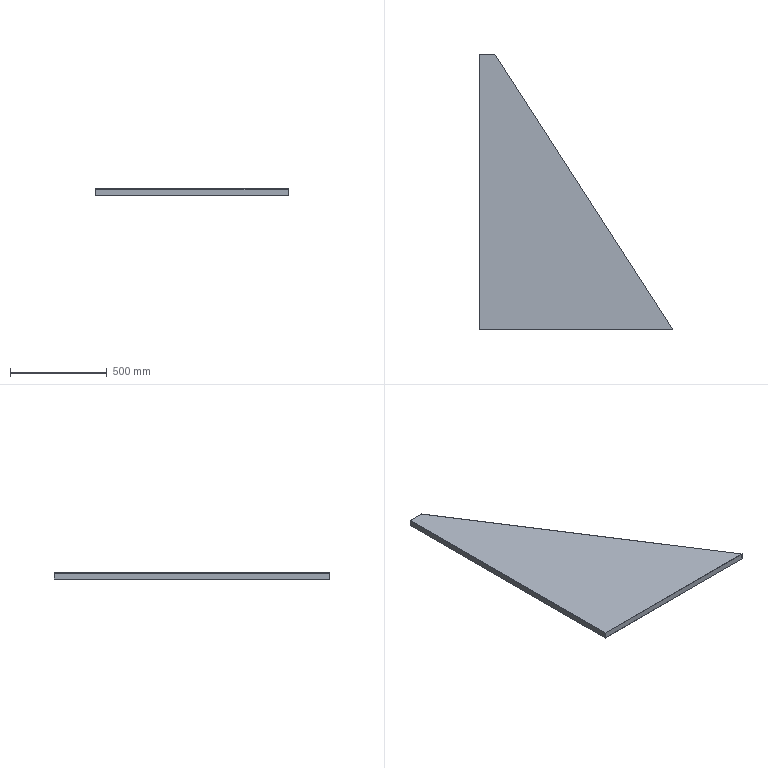Part | SolidWorks | features ICE 2, Extrusion 1 | 1 solid | 12 faces | box 1002 x 1427 x 32 mm | volume 1793698 mm3 | plane 12
STEP:
#1=CARTESIAN_POINT('',(-501.,713.5,0.));
#2=VERTEX_POINT('',#1);
#3=CARTESIAN_POINT('',(-499.,711.5,0.));
#4=VERTEX_POINT('',#3);
#5=CARTESIAN_POINT('',(-501.,713.5,0.));
#6=DIRECTION('',(0.7071,-0.7071,0.));
#7=VECTOR('',#6,1000.);
#8=LINE('',#5,#7);
#9=EDGE_CURVE('',#2,#4,#8,.T.);
#10=ORIENTED_EDGE('',*,*,#9,.F.);
#11=CARTESIAN_POINT('',(-419.25,713.5,0.));
#12=VERTEX_POINT('',#11);
#13=CARTESIAN_POINT('',(-501.,713.5,0.));
#14=DIRECTION('',(-1.,0.,0.));
#15=VECTOR('',#14,1000.);
#16=LINE('',#13,#15);
#17=EDGE_CURVE('',#12,#2,#16,.T.);
#18=ORIENTED_EDGE('',*,*,#17,.F.);
#19=CARTESIAN_POINT('',(-420.34,711.5,0.));
#20=VERTEX_POINT('',#19);
#21=CARTESIAN_POINT('',(-419.25,713.5,0.));
#22=DIRECTION('',(0.4786,0.8781,0.));
#23=VECTOR('',#22,1000.);
#24=LINE('',#21,#23);
#25=EDGE_CURVE('',#20,#12,#24,.T.);
#26=ORIENTED_EDGE('',*,*,#25,.F.);
#27=CARTESIAN_POINT('',(497.33,-711.5,0.));
#28=VERTEX_POINT('',#27);
#29=CARTESIAN_POINT('',(-420.34,711.5,0.));
#30=DIRECTION('',(-0.542,0.8404,0.));
#31=VECTOR('',#30,1000.);
#32=LINE('',#29,#31);
#33=EDGE_CURVE('',#28,#20,#32,.T.);
#34=ORIENTED_EDGE('',*,*,#33,.F.);
#35=CARTESIAN_POINT('',(-499.,-711.5,0.));
#36=VERTEX_POINT('',#35);
#37=CARTESIAN_POINT('',(497.33,-711.5,0.));
#38=DIRECTION('',(1.,0.,0.));
#39=VECTOR('',#38,1000.);
#40=LINE('',#37,#39);
#41=EDGE_CURVE('',#36,#28,#40,.T.);
#42=ORIENTED_EDGE('',*,*,#41,.F.);
#43=CARTESIAN_POINT('',(-499.,-711.5,0.));
#44=DIRECTION('',(0.,-1.,0.));
#45=VECTOR('',#44,1000.);
#46=LINE('',#43,#45);
#47=EDGE_CURVE('',#4,#36,#46,.T.);
#48=ORIENTED_EDGE('',*,*,#47,.F.);
#49=EDGE_LOOP('',(#10,#18,#26,#34,#42,#48));
#50=FACE_OUTER_BOUND('',#49,.T.);
#51=CARTESIAN_POINT('',(0.,0.,0.));
#52=DIRECTION('',(0.,0.,1.));
#53=DIRECTION('',(1.,0.,0.));
#54=AXIS2_PLACEMENT_3D('',#51,#52,#53);
#55=PLANE('',#54);
#56=ADVANCED_FACE('',(#50),#55,.F.);
#57=CARTESIAN_POINT('',(-419.25,713.5,2.));
#58=VERTEX_POINT('',#57);
#59=CARTESIAN_POINT('',(-501.,713.5,2.));
#60=VERTEX_POINT('',#59);
#61=CARTESIAN_POINT('',(-501.,713.5,2.));
#62=DIRECTION('',(-1.,0.,0.));
#63=VECTOR('',#62,1000.);
#64=LINE('',#61,#63);
#65=EDGE_CURVE('',#58,#60,#64,.T.);
#66=ORIENTED_EDGE('',*,*,#65,.F.);
#67=CARTESIAN_POINT('',(-419.25,713.5,0.));
#68=DIRECTION('',(0.,0.,1.));
#69=VECTOR('',#68,1000.);
#70=LINE('',#67,#69);
#71=EDGE_CURVE('',#12,#58,#70,.T.);
#72=ORIENTED_EDGE('',*,*,#71,.F.);
#73=ORIENTED_EDGE('',*,*,#17,.T.);
#74=CARTESIAN_POINT('',(-501.,713.5,2.));
#75=DIRECTION('',(0.,0.,-1.));
#76=VECTOR('',#75,1000.);
#77=LINE('',#74,#76);
#78=EDGE_CURVE('',#60,#2,#77,.T.);
#79=ORIENTED_EDGE('',*,*,#78,.F.);
#80=EDGE_LOOP('',(#66,#72,#73,#79));
#81=FACE_OUTER_BOUND('',#80,.T.);
#82=CARTESIAN_POINT('',(-501.,713.5,2.));
#83=DIRECTION('',(0.,-1.,0.));
#84=DIRECTION('',(0.,0.,-1.));
#85=AXIS2_PLACEMENT_3D('',#82,#83,#84);
#86=PLANE('',#85);
#87=ADVANCED_FACE('',(#81),#86,.F.);
#88=ORIENTED_EDGE('',*,*,#78,.T.);
#89=CARTESIAN_POINT('',(-501.,713.5,-30.));
#90=VERTEX_POINT('',#89);
#91=CARTESIAN_POINT('',(-501.,713.5,-30.));
#92=DIRECTION('',(0.,0.,1.));
#93=VECTOR('',#92,1000.);
#94=LINE('',#91,#93);
#95=EDGE_CURVE('',#90,#2,#94,.T.);
#96=ORIENTED_EDGE('',*,*,#95,.F.);
#97=CARTESIAN_POINT('',(-501.,-713.5,-30.));
#98=VERTEX_POINT('',#97);
#99=CARTESIAN_POINT('',(-501.,-713.5,-30.));
#100=DIRECTION('',(0.,1.,0.));
#101=VECTOR('',#100,1000.);
#102=LINE('',#99,#101);
#103=EDGE_CURVE('',#98,#90,#102,.T.);
#104=ORIENTED_EDGE('',*,*,#103,.F.);
#105=CARTESIAN_POINT('',(-501.,-713.5,2.));
#106=VERTEX_POINT('',#105);
#107=CARTESIAN_POINT('',(-501.,-713.5,2.));
#108=DIRECTION('',(0.,0.,-1.));
#109=VECTOR('',#108,1000.);
#110=LINE('',#107,#109);
#111=EDGE_CURVE('',#106,#98,#110,.T.);
#112=ORIENTED_EDGE('',*,*,#111,.F.);
#113=CARTESIAN_POINT('',(-501.,713.5,2.));
#114=DIRECTION('',(0.,-1.,0.));
#115=VECTOR('',#114,1000.);
#116=LINE('',#113,#115);
#117=EDGE_CURVE('',#60,#106,#116,.T.);
#118=ORIENTED_EDGE('',*,*,#117,.F.);
#119=EDGE_LOOP('',(#88,#96,#104,#112,#118));
#120=FACE_OUTER_BOUND('',#119,.T.);
#121=CARTESIAN_POINT('',(-501.,713.5,2.));
#122=DIRECTION('',(1.,0.,0.));
#123=DIRECTION('',(0.,1.,0.));
#124=AXIS2_PLACEMENT_3D('',#121,#122,#123);
#125=PLANE('',#124);
#126=ADVANCED_FACE('',(#120),#125,.F.);
#127=ORIENTED_EDGE('',*,*,#111,.T.);
#128=CARTESIAN_POINT('',(501.,-713.5,-30.));
#129=VERTEX_POINT('',#128);
#130=CARTESIAN_POINT('',(501.,-713.5,-30.));
#131=DIRECTION('',(-1.,0.,0.));
#132=VECTOR('',#131,1000.);
#133=LINE('',#130,#132);
#134=EDGE_CURVE('',#129,#98,#133,.T.);
#135=ORIENTED_EDGE('',*,*,#134,.F.);
#136=CARTESIAN_POINT('',(501.,-713.5,2.));
#137=VERTEX_POINT('',#136);
#138=CARTESIAN_POINT('',(501.,-713.5,2.));
#139=DIRECTION('',(0.,0.,-1.));
#140=VECTOR('',#139,1000.);
#141=LINE('',#138,#140);
#142=EDGE_CURVE('',#137,#129,#141,.T.);
#143=ORIENTED_EDGE('',*,*,#142,.F.);
#144=CARTESIAN_POINT('',(-501.,-713.5,2.));
#145=DIRECTION('',(1.,0.,0.));
#146=VECTOR('',#145,1000.);
#147=LINE('',#144,#146);
#148=EDGE_CURVE('',#106,#137,#147,.T.);
#149=ORIENTED_EDGE('',*,*,#148,.F.);
#150=EDGE_LOOP('',(#127,#135,#143,#149));
#151=FACE_OUTER_BOUND('',#150,.T.);
#152=CARTESIAN_POINT('',(-501.,-713.5,2.));
#153=DIRECTION('',(0.,1.,0.));
#154=DIRECTION('',(0.,0.,1.));
#155=AXIS2_PLACEMENT_3D('',#152,#153,#154);
#156=PLANE('',#155);
#157=ADVANCED_FACE('',(#151),#156,.F.);
#158=CARTESIAN_POINT('',(-419.25,713.5,2.));
#159=DIRECTION('',(0.542,-0.8404,0.));
#160=VECTOR('',#159,1000.);
#161=LINE('',#158,#160);
#162=EDGE_CURVE('',#58,#137,#161,.T.);
#163=ORIENTED_EDGE('',*,*,#162,.F.);
#164=ORIENTED_EDGE('',*,*,#65,.T.);
#165=ORIENTED_EDGE('',*,*,#117,.T.);
#166=ORIENTED_EDGE('',*,*,#148,.T.);
#167=EDGE_LOOP('',(#163,#164,#165,#166));
#168=FACE_OUTER_BOUND('',#167,.T.);
#169=CARTESIAN_POINT('',(0.,0.,2.));
#170=DIRECTION('',(0.,0.,1.));
#171=DIRECTION('',(1.,0.,0.));
#172=AXIS2_PLACEMENT_3D('',#169,#170,#171);
#173=PLANE('',#172);
#174=ADVANCED_FACE('',(#168),#173,.T.);
#175=ORIENTED_EDGE('',*,*,#162,.T.);
#176=ORIENTED_EDGE('',*,*,#142,.T.);
#177=CARTESIAN_POINT('',(-419.25,713.5,-30.));
#178=VERTEX_POINT('',#177);
#179=CARTESIAN_POINT('',(-419.25,713.5,-30.));
#180=DIRECTION('',(0.542,-0.8404,0.));
#181=VECTOR('',#180,1000.);
#182=LINE('',#179,#181);
#183=EDGE_CURVE('',#178,#129,#182,.T.);
#184=ORIENTED_EDGE('',*,*,#183,.F.);
#185=CARTESIAN_POINT('',(-419.25,713.5,-30.));
#186=DIRECTION('',(0.,0.,1.));
#187=VECTOR('',#186,1000.);
#188=LINE('',#185,#187);
#189=EDGE_CURVE('',#178,#12,#188,.T.);
#190=ORIENTED_EDGE('',*,*,#189,.T.);
#191=ORIENTED_EDGE('',*,*,#71,.T.);
#192=EDGE_LOOP('',(#175,#176,#184,#190,#191));
#193=FACE_OUTER_BOUND('',#192,.T.);
#194=CARTESIAN_POINT('',(-419.25,713.5,0.));
#195=DIRECTION('',(-0.8404,-0.542,0.));
#196=DIRECTION('',(0.542,-0.8404,0.));
#197=AXIS2_PLACEMENT_3D('',#194,#195,#196);
#198=PLANE('',#197);
#199=ADVANCED_FACE('',(#193),#198,.F.);
#200=ORIENTED_EDGE('',*,*,#9,.T.);
#201=CARTESIAN_POINT('',(-499.,711.5,-30.));
#202=VERTEX_POINT('',#201);
#203=CARTESIAN_POINT('',(-499.,711.5,-30.));
#204=DIRECTION('',(0.,0.,1.));
#205=VECTOR('',#204,1000.);
#206=LINE('',#203,#205);
#207=EDGE_CURVE('',#202,#4,#206,.T.);
#208=ORIENTED_EDGE('',*,*,#207,.F.);
#209=CARTESIAN_POINT('',(-501.,713.5,-30.));
#210=DIRECTION('',(0.7071,-0.7071,0.));
#211=VECTOR('',#210,1000.);
#212=LINE('',#209,#211);
#213=EDGE_CURVE('',#90,#202,#212,.T.);
#214=ORIENTED_EDGE('',*,*,#213,.F.);
#215=ORIENTED_EDGE('',*,*,#95,.T.);
#216=EDGE_LOOP('',(#200,#208,#214,#215));
#217=FACE_OUTER_BOUND('',#216,.T.);
#218=CARTESIAN_POINT('',(-501.,713.5,-30.));
#219=DIRECTION('',(-0.7071,-0.7071,0.));
#220=DIRECTION('',(0.7071,-0.7071,0.));
#221=AXIS2_PLACEMENT_3D('',#218,#219,#220);
#222=PLANE('',#221);
#223=ADVANCED_FACE('',(#217),#222,.F.);
#224=ORIENTED_EDGE('',*,*,#47,.T.);
#225=CARTESIAN_POINT('',(-499.,-711.5,-30.));
#226=VERTEX_POINT('',#225);
#227=CARTESIAN_POINT('',(-499.,-711.5,-30.));
#228=DIRECTION('',(0.,0.,1.));
#229=VECTOR('',#228,1000.);
#230=LINE('',#227,#229);
#231=EDGE_CURVE('',#226,#36,#230,.T.);
#232=ORIENTED_EDGE('',*,*,#231,.F.);
#233=CARTESIAN_POINT('',(-499.,-711.5,-30.));
#234=DIRECTION('',(0.,-1.,0.));
#235=VECTOR('',#234,1000.);
#236=LINE('',#233,#235);
#237=EDGE_CURVE('',#202,#226,#236,.T.);
#238=ORIENTED_EDGE('',*,*,#237,.F.);
#239=ORIENTED_EDGE('',*,*,#207,.T.);
#240=EDGE_LOOP('',(#224,#232,#238,#239));
#241=FACE_OUTER_BOUND('',#240,.T.);
#242=CARTESIAN_POINT('',(-499.,-711.5,-30.));
#243=DIRECTION('',(-1.,0.,0.));
#244=DIRECTION('',(0.,0.,1.));
#245=AXIS2_PLACEMENT_3D('',#242,#243,#244);
#246=PLANE('',#245);
#247=ADVANCED_FACE('',(#241),#246,.F.);
#248=ORIENTED_EDGE('',*,*,#41,.T.);
#249=CARTESIAN_POINT('',(497.33,-711.5,-30.));
#250=VERTEX_POINT('',#249);
#251=CARTESIAN_POINT('',(497.33,-711.5,-30.));
#252=DIRECTION('',(0.,0.,1.));
#253=VECTOR('',#252,1000.);
#254=LINE('',#251,#253);
#255=EDGE_CURVE('',#250,#28,#254,.T.);
#256=ORIENTED_EDGE('',*,*,#255,.F.);
#257=CARTESIAN_POINT('',(497.33,-711.5,-30.));
#258=DIRECTION('',(1.,0.,0.));
#259=VECTOR('',#258,1000.);
#260=LINE('',#257,#259);
#261=EDGE_CURVE('',#226,#250,#260,.T.);
#262=ORIENTED_EDGE('',*,*,#261,.F.);
#263=ORIENTED_EDGE('',*,*,#231,.T.);
#264=EDGE_LOOP('',(#248,#256,#262,#263));
#265=FACE_OUTER_BOUND('',#264,.T.);
#266=CARTESIAN_POINT('',(497.33,-711.5,-30.));
#267=DIRECTION('',(0.,-1.,0.));
#268=DIRECTION('',(1.,0.,0.));
#269=AXIS2_PLACEMENT_3D('',#266,#267,#268);
#270=PLANE('',#269);
#271=ADVANCED_FACE('',(#265),#270,.F.);
#272=ORIENTED_EDGE('',*,*,#33,.T.);
#273=CARTESIAN_POINT('',(-420.34,711.5,-30.));
#274=VERTEX_POINT('',#273);
#275=CARTESIAN_POINT('',(-420.34,711.5,-30.));
#276=DIRECTION('',(0.,0.,1.));
#277=VECTOR('',#276,1000.);
#278=LINE('',#275,#277);
#279=EDGE_CURVE('',#274,#20,#278,.T.);
#280=ORIENTED_EDGE('',*,*,#279,.F.);
#281=CARTESIAN_POINT('',(-420.34,711.5,-30.));
#282=DIRECTION('',(-0.542,0.8404,0.));
#283=VECTOR('',#282,1000.);
#284=LINE('',#281,#283);
#285=EDGE_CURVE('',#250,#274,#284,.T.);
#286=ORIENTED_EDGE('',*,*,#285,.F.);
#287=ORIENTED_EDGE('',*,*,#255,.T.);
#288=EDGE_LOOP('',(#272,#280,#286,#287));
#289=FACE_OUTER_BOUND('',#288,.T.);
#290=CARTESIAN_POINT('',(-420.34,711.5,-30.));
#291=DIRECTION('',(0.8404,0.542,0.));
#292=DIRECTION('',(-0.542,0.8404,0.));
#293=AXIS2_PLACEMENT_3D('',#290,#291,#292);
#294=PLANE('',#293);
#295=ADVANCED_FACE('',(#289),#294,.F.);
#296=ORIENTED_EDGE('',*,*,#25,.T.);
#297=ORIENTED_EDGE('',*,*,#189,.F.);
#298=CARTESIAN_POINT('',(-419.25,713.5,-30.));
#299=DIRECTION('',(0.4786,0.8781,0.));
#300=VECTOR('',#299,1000.);
#301=LINE('',#298,#300);
#302=EDGE_CURVE('',#274,#178,#301,.T.);
#303=ORIENTED_EDGE('',*,*,#302,.F.);
#304=ORIENTED_EDGE('',*,*,#279,.T.);
#305=EDGE_LOOP('',(#296,#297,#303,#304));
#306=FACE_OUTER_BOUND('',#305,.T.);
#307=CARTESIAN_POINT('',(-419.25,713.5,-30.));
#308=DIRECTION('',(0.8781,-0.4786,0.));
#309=DIRECTION('',(0.4786,0.8781,0.));
#310=AXIS2_PLACEMENT_3D('',#307,#308,#309);
#311=PLANE('',#310);
#312=ADVANCED_FACE('',(#306),#311,.F.);
#313=ORIENTED_EDGE('',*,*,#213,.T.);
#314=ORIENTED_EDGE('',*,*,#237,.T.);
#315=ORIENTED_EDGE('',*,*,#261,.T.);
#316=ORIENTED_EDGE('',*,*,#285,.T.);
#317=ORIENTED_EDGE('',*,*,#302,.T.);
#318=ORIENTED_EDGE('',*,*,#183,.T.);
#319=ORIENTED_EDGE('',*,*,#134,.T.);
#320=ORIENTED_EDGE('',*,*,#103,.T.);
#321=EDGE_LOOP('',(#313,#314,#315,#316,#317,#318,#319,#320));
#322=FACE_OUTER_BOUND('',#321,.T.);
#323=CARTESIAN_POINT('',(0.,0.,-30.));
#324=DIRECTION('',(0.,0.,-1.));
#325=DIRECTION('',(-1.,0.,0.));
#326=AXIS2_PLACEMENT_3D('',#323,#324,#325);
#327=PLANE('',#326);
#328=ADVANCED_FACE('',(#322),#327,.T.);
#329=CLOSED_SHELL('',(#56,#87,#126,#157,#174,#199,#223,#247,#271,#295,#312,#328));
#330=MANIFOLD_SOLID_BREP('',#329);
#331=CARTESIAN_POINT('',(0.,0.,0.));
#332=DIRECTION('',(0.,0.,1.));
#333=DIRECTION('',(1.,0.,0.));
#334=AXIS2_PLACEMENT_3D('',#331,#332,#333);
#335=(LENGTH_UNIT()NAMED_UNIT(*)SI_UNIT(.MILLI.,.METRE.));
#336=UNCERTAINTY_MEASURE_WITH_UNIT(LENGTH_MEASURE(0.00001),#335,'','');
#337=(NAMED_UNIT(*)PLANE_ANGLE_UNIT()SI_UNIT($,.RADIAN.));
#338=(NAMED_UNIT(*)SI_UNIT($,.STERADIAN.)SOLID_ANGLE_UNIT());
#339=(GEOMETRIC_REPRESENTATION_CONTEXT(3)GLOBAL_UNCERTAINTY_ASSIGNED_CONTEXT((#336))GLOBAL_UNIT_ASSIGNED_CONTEXT((#335,#337,#338))REPRESENTATION_CONTEXT('',''));
#340=ADVANCED_BREP_SHAPE_REPRESENTATION('',(#330,#334),#339);